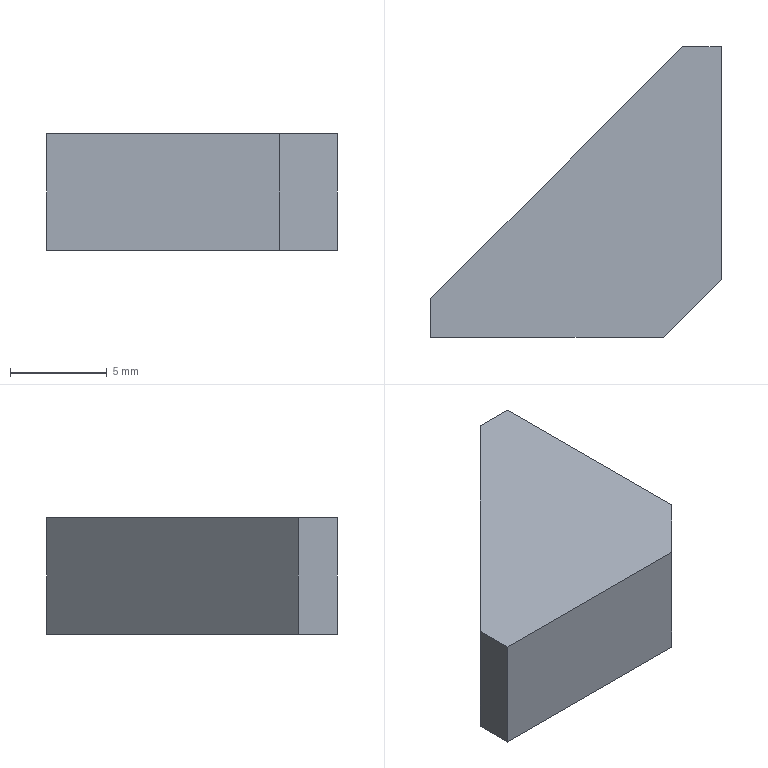Part | SolidWorks | features FlatPattern 1, SMBaseFlange 1, SheetMetal 1 | 1 solid | 8 faces | box 15 x 15 x 6 mm | volume 816 mm3 | plane 8
STEP:
#1=CARTESIAN_POINT('',(0.,2.,0.));
#2=VERTEX_POINT('',#1);
#3=CARTESIAN_POINT('',(0.,0.,0.));
#4=VERTEX_POINT('',#3);
#5=CARTESIAN_POINT('',(0.,2.,0.));
#6=DIRECTION('',(0.,-1.,0.));
#7=VECTOR('',#6,1000.);
#8=LINE('',#5,#7);
#9=EDGE_CURVE('',#2,#4,#8,.T.);
#10=ORIENTED_EDGE('',*,*,#9,.F.);
#11=CARTESIAN_POINT('',(0.,2.,-6.));
#12=VERTEX_POINT('',#11);
#13=CARTESIAN_POINT('',(0.,2.,-6.));
#14=DIRECTION('',(0.,0.,1.));
#15=VECTOR('',#14,1000.);
#16=LINE('',#13,#15);
#17=EDGE_CURVE('',#12,#2,#16,.T.);
#18=ORIENTED_EDGE('',*,*,#17,.F.);
#19=CARTESIAN_POINT('',(0.,0.,-6.));
#20=VERTEX_POINT('',#19);
#21=CARTESIAN_POINT('',(0.,2.,-6.));
#22=DIRECTION('',(0.,-1.,0.));
#23=VECTOR('',#22,1000.);
#24=LINE('',#21,#23);
#25=EDGE_CURVE('',#12,#20,#24,.T.);
#26=ORIENTED_EDGE('',*,*,#25,.T.);
#27=CARTESIAN_POINT('',(0.,0.,-6.));
#28=DIRECTION('',(0.,0.,1.));
#29=VECTOR('',#28,1000.);
#30=LINE('',#27,#29);
#31=EDGE_CURVE('',#20,#4,#30,.T.);
#32=ORIENTED_EDGE('',*,*,#31,.T.);
#33=EDGE_LOOP('',(#10,#18,#26,#32));
#34=FACE_OUTER_BOUND('',#33,.T.);
#35=CARTESIAN_POINT('',(0.,2.,-6.));
#36=DIRECTION('',(-1.,0.,0.));
#37=DIRECTION('',(0.,-1.,0.));
#38=AXIS2_PLACEMENT_3D('',#35,#36,#37);
#39=PLANE('',#38);
#40=ADVANCED_FACE('',(#34),#39,.T.);
#41=CARTESIAN_POINT('',(13.,15.,0.));
#42=VERTEX_POINT('',#41);
#43=CARTESIAN_POINT('',(13.,15.,0.));
#44=DIRECTION('',(-0.7071,-0.7071,0.));
#45=VECTOR('',#44,1000.);
#46=LINE('',#43,#45);
#47=EDGE_CURVE('',#42,#2,#46,.T.);
#48=ORIENTED_EDGE('',*,*,#47,.F.);
#49=CARTESIAN_POINT('',(13.,15.,-6.));
#50=VERTEX_POINT('',#49);
#51=CARTESIAN_POINT('',(13.,15.,-6.));
#52=DIRECTION('',(0.,0.,1.));
#53=VECTOR('',#52,1000.);
#54=LINE('',#51,#53);
#55=EDGE_CURVE('',#50,#42,#54,.T.);
#56=ORIENTED_EDGE('',*,*,#55,.F.);
#57=CARTESIAN_POINT('',(13.,15.,-6.));
#58=DIRECTION('',(-0.7071,-0.7071,0.));
#59=VECTOR('',#58,1000.);
#60=LINE('',#57,#59);
#61=EDGE_CURVE('',#50,#12,#60,.T.);
#62=ORIENTED_EDGE('',*,*,#61,.T.);
#63=ORIENTED_EDGE('',*,*,#17,.T.);
#64=EDGE_LOOP('',(#48,#56,#62,#63));
#65=FACE_OUTER_BOUND('',#64,.T.);
#66=CARTESIAN_POINT('',(13.,15.,-6.));
#67=DIRECTION('',(-0.7071,0.7071,0.));
#68=DIRECTION('',(-0.7071,-0.7071,0.));
#69=AXIS2_PLACEMENT_3D('',#66,#67,#68);
#70=PLANE('',#69);
#71=ADVANCED_FACE('',(#65),#70,.T.);
#72=CARTESIAN_POINT('',(15.,15.,0.));
#73=VERTEX_POINT('',#72);
#74=CARTESIAN_POINT('',(15.,15.,0.));
#75=DIRECTION('',(-1.,0.,0.));
#76=VECTOR('',#75,1000.);
#77=LINE('',#74,#76);
#78=EDGE_CURVE('',#73,#42,#77,.T.);
#79=ORIENTED_EDGE('',*,*,#78,.F.);
#80=CARTESIAN_POINT('',(15.,15.,-6.));
#81=VERTEX_POINT('',#80);
#82=CARTESIAN_POINT('',(15.,15.,-6.));
#83=DIRECTION('',(0.,0.,1.));
#84=VECTOR('',#83,1000.);
#85=LINE('',#82,#84);
#86=EDGE_CURVE('',#81,#73,#85,.T.);
#87=ORIENTED_EDGE('',*,*,#86,.F.);
#88=CARTESIAN_POINT('',(15.,15.,-6.));
#89=DIRECTION('',(-1.,0.,0.));
#90=VECTOR('',#89,1000.);
#91=LINE('',#88,#90);
#92=EDGE_CURVE('',#81,#50,#91,.T.);
#93=ORIENTED_EDGE('',*,*,#92,.T.);
#94=ORIENTED_EDGE('',*,*,#55,.T.);
#95=EDGE_LOOP('',(#79,#87,#93,#94));
#96=FACE_OUTER_BOUND('',#95,.T.);
#97=CARTESIAN_POINT('',(15.,15.,-6.));
#98=DIRECTION('',(0.,1.,0.));
#99=DIRECTION('',(0.,0.,1.));
#100=AXIS2_PLACEMENT_3D('',#97,#98,#99);
#101=PLANE('',#100);
#102=ADVANCED_FACE('',(#96),#101,.T.);
#103=CARTESIAN_POINT('',(15.,3.,0.));
#104=VERTEX_POINT('',#103);
#105=CARTESIAN_POINT('',(15.,3.,0.));
#106=DIRECTION('',(0.,1.,0.));
#107=VECTOR('',#106,1000.);
#108=LINE('',#105,#107);
#109=EDGE_CURVE('',#104,#73,#108,.T.);
#110=ORIENTED_EDGE('',*,*,#109,.F.);
#111=CARTESIAN_POINT('',(15.,3.,-6.));
#112=VERTEX_POINT('',#111);
#113=CARTESIAN_POINT('',(15.,3.,-6.));
#114=DIRECTION('',(0.,0.,1.));
#115=VECTOR('',#114,1000.);
#116=LINE('',#113,#115);
#117=EDGE_CURVE('',#112,#104,#116,.T.);
#118=ORIENTED_EDGE('',*,*,#117,.F.);
#119=CARTESIAN_POINT('',(15.,3.,-6.));
#120=DIRECTION('',(0.,1.,0.));
#121=VECTOR('',#120,1000.);
#122=LINE('',#119,#121);
#123=EDGE_CURVE('',#112,#81,#122,.T.);
#124=ORIENTED_EDGE('',*,*,#123,.T.);
#125=ORIENTED_EDGE('',*,*,#86,.T.);
#126=EDGE_LOOP('',(#110,#118,#124,#125));
#127=FACE_OUTER_BOUND('',#126,.T.);
#128=CARTESIAN_POINT('',(15.,3.,-6.));
#129=DIRECTION('',(1.,0.,0.));
#130=DIRECTION('',(0.,0.,-1.));
#131=AXIS2_PLACEMENT_3D('',#128,#129,#130);
#132=PLANE('',#131);
#133=ADVANCED_FACE('',(#127),#132,.T.);
#134=CARTESIAN_POINT('',(12.,0.,0.));
#135=VERTEX_POINT('',#134);
#136=CARTESIAN_POINT('',(12.,0.,0.));
#137=DIRECTION('',(0.7071,0.7071,0.));
#138=VECTOR('',#137,1000.);
#139=LINE('',#136,#138);
#140=EDGE_CURVE('',#135,#104,#139,.T.);
#141=ORIENTED_EDGE('',*,*,#140,.F.);
#142=CARTESIAN_POINT('',(12.,0.,-6.));
#143=VERTEX_POINT('',#142);
#144=CARTESIAN_POINT('',(12.,0.,-6.));
#145=DIRECTION('',(0.,0.,1.));
#146=VECTOR('',#145,1000.);
#147=LINE('',#144,#146);
#148=EDGE_CURVE('',#143,#135,#147,.T.);
#149=ORIENTED_EDGE('',*,*,#148,.F.);
#150=CARTESIAN_POINT('',(12.,0.,-6.));
#151=DIRECTION('',(0.7071,0.7071,0.));
#152=VECTOR('',#151,1000.);
#153=LINE('',#150,#152);
#154=EDGE_CURVE('',#143,#112,#153,.T.);
#155=ORIENTED_EDGE('',*,*,#154,.T.);
#156=ORIENTED_EDGE('',*,*,#117,.T.);
#157=EDGE_LOOP('',(#141,#149,#155,#156));
#158=FACE_OUTER_BOUND('',#157,.T.);
#159=CARTESIAN_POINT('',(12.,0.,-6.));
#160=DIRECTION('',(0.7071,-0.7071,0.));
#161=DIRECTION('',(0.7071,0.7071,0.));
#162=AXIS2_PLACEMENT_3D('',#159,#160,#161);
#163=PLANE('',#162);
#164=ADVANCED_FACE('',(#158),#163,.T.);
#165=CARTESIAN_POINT('',(0.,0.,0.));
#166=DIRECTION('',(1.,0.,0.));
#167=VECTOR('',#166,1000.);
#168=LINE('',#165,#167);
#169=EDGE_CURVE('',#4,#135,#168,.T.);
#170=ORIENTED_EDGE('',*,*,#169,.F.);
#171=ORIENTED_EDGE('',*,*,#31,.F.);
#172=CARTESIAN_POINT('',(0.,0.,-6.));
#173=DIRECTION('',(1.,0.,0.));
#174=VECTOR('',#173,1000.);
#175=LINE('',#172,#174);
#176=EDGE_CURVE('',#20,#143,#175,.T.);
#177=ORIENTED_EDGE('',*,*,#176,.T.);
#178=ORIENTED_EDGE('',*,*,#148,.T.);
#179=EDGE_LOOP('',(#170,#171,#177,#178));
#180=FACE_OUTER_BOUND('',#179,.T.);
#181=CARTESIAN_POINT('',(0.,0.,-6.));
#182=DIRECTION('',(0.,-1.,0.));
#183=DIRECTION('',(0.,0.,-1.));
#184=AXIS2_PLACEMENT_3D('',#181,#182,#183);
#185=PLANE('',#184);
#186=ADVANCED_FACE('',(#180),#185,.T.);
#187=ORIENTED_EDGE('',*,*,#25,.F.);
#188=ORIENTED_EDGE('',*,*,#61,.F.);
#189=ORIENTED_EDGE('',*,*,#92,.F.);
#190=ORIENTED_EDGE('',*,*,#123,.F.);
#191=ORIENTED_EDGE('',*,*,#154,.F.);
#192=ORIENTED_EDGE('',*,*,#176,.F.);
#193=EDGE_LOOP('',(#187,#188,#189,#190,#191,#192));
#194=FACE_OUTER_BOUND('',#193,.T.);
#195=CARTESIAN_POINT('',(0.,0.,-6.));
#196=DIRECTION('',(0.,0.,1.));
#197=DIRECTION('',(1.,0.,0.));
#198=AXIS2_PLACEMENT_3D('',#195,#196,#197);
#199=PLANE('',#198);
#200=ADVANCED_FACE('',(#194),#199,.F.);
#201=ORIENTED_EDGE('',*,*,#9,.T.);
#202=ORIENTED_EDGE('',*,*,#169,.T.);
#203=ORIENTED_EDGE('',*,*,#140,.T.);
#204=ORIENTED_EDGE('',*,*,#109,.T.);
#205=ORIENTED_EDGE('',*,*,#78,.T.);
#206=ORIENTED_EDGE('',*,*,#47,.T.);
#207=EDGE_LOOP('',(#201,#202,#203,#204,#205,#206));
#208=FACE_OUTER_BOUND('',#207,.T.);
#209=CARTESIAN_POINT('',(0.,0.,0.));
#210=DIRECTION('',(0.,0.,1.));
#211=DIRECTION('',(1.,0.,0.));
#212=AXIS2_PLACEMENT_3D('',#209,#210,#211);
#213=PLANE('',#212);
#214=ADVANCED_FACE('',(#208),#213,.T.);
#215=CLOSED_SHELL('',(#40,#71,#102,#133,#164,#186,#200,#214));
#216=MANIFOLD_SOLID_BREP('',#215);
#217=CARTESIAN_POINT('',(0.,0.,0.));
#218=DIRECTION('',(0.,0.,1.));
#219=DIRECTION('',(1.,0.,0.));
#220=AXIS2_PLACEMENT_3D('',#217,#218,#219);
#221=(LENGTH_UNIT()NAMED_UNIT(*)SI_UNIT(.MILLI.,.METRE.));
#222=UNCERTAINTY_MEASURE_WITH_UNIT(LENGTH_MEASURE(0.00001),#221,'','');
#223=(NAMED_UNIT(*)PLANE_ANGLE_UNIT()SI_UNIT($,.RADIAN.));
#224=(NAMED_UNIT(*)SI_UNIT($,.STERADIAN.)SOLID_ANGLE_UNIT());
#225=(GEOMETRIC_REPRESENTATION_CONTEXT(3)GLOBAL_UNCERTAINTY_ASSIGNED_CONTEXT((#222))GLOBAL_UNIT_ASSIGNED_CONTEXT((#221,#223,#224))REPRESENTATION_CONTEXT('',''));
#226=ADVANCED_BREP_SHAPE_REPRESENTATION('',(#216,#220),#225);